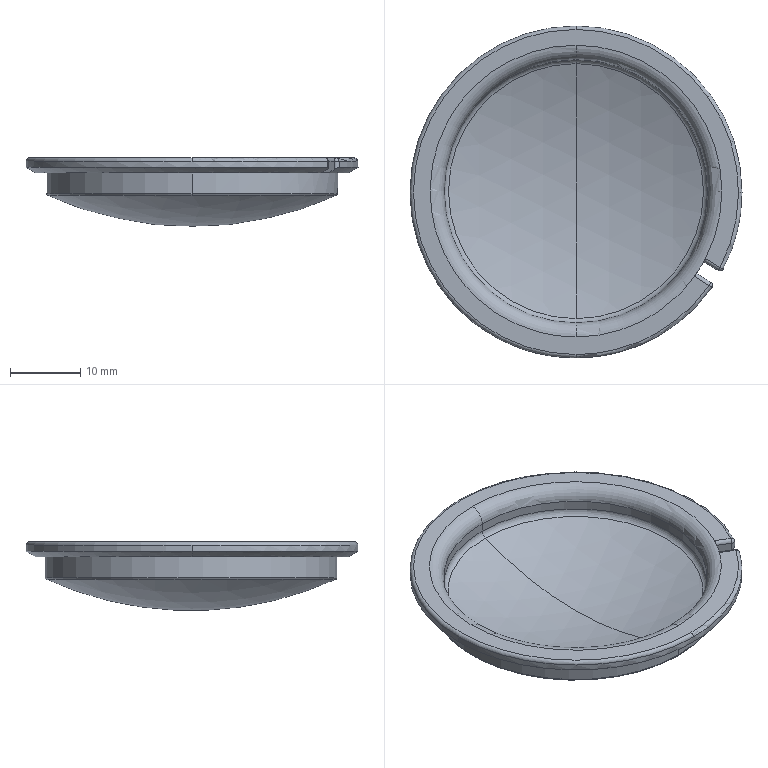Part | SolidWorks | features BaseBody 1 | 1 solid | 32 faces | box 47.34 x 47.34 x 9.8 mm | volume 4402 mm3 | torus 12 | cylinder 11 | sphere 5 | plane 4 | commonest cylinder face diameters 1 x4 47.34 x3 37.6 x2 41.6 x2
STEP:
#1=CARTESIAN_POINT('',(-125.381,28.46,-0.4856));
#2=VERTEX_POINT('',#1);
#3=CARTESIAN_POINT('',(-125.381,-12.906,-0.4856));
#4=VERTEX_POINT('',#3);
#5=CARTESIAN_POINT('',(-125.381,7.777,-0.4856));
#6=DIRECTION('',(0.,0.,-1.));
#7=DIRECTION('',(0.,-1.,0.));
#8=AXIS2_PLACEMENT_3D('',#5,#6,#7);
#9=CIRCLE('',#8,20.683);
#10=EDGE_CURVE('',#2,#4,#9,.T.);
#11=ORIENTED_EDGE('',*,*,#10,.F.);
#12=CARTESIAN_POINT('',(-125.381,28.577,-0.3035));
#13=VERTEX_POINT('',#12);
#14=CARTESIAN_POINT('',(-125.381,28.377,-0.3035));
#15=DIRECTION('',(1.,0.,0.));
#16=DIRECTION('',(0.,1.,0.));
#17=AXIS2_PLACEMENT_3D('',#14,#15,#16);
#18=CIRCLE('',#17,0.2);
#19=EDGE_CURVE('',#2,#13,#18,.T.);
#20=ORIENTED_EDGE('',*,*,#19,.T.);
#21=CARTESIAN_POINT('',(-125.381,-13.023,-0.3035));
#22=VERTEX_POINT('',#21);
#23=CARTESIAN_POINT('',(-125.381,7.777,-0.3035));
#24=DIRECTION('',(0.,0.,-1.));
#25=DIRECTION('',(0.,1.,0.));
#26=AXIS2_PLACEMENT_3D('',#23,#24,#25);
#27=CIRCLE('',#26,20.8);
#28=EDGE_CURVE('',#13,#22,#27,.T.);
#29=ORIENTED_EDGE('',*,*,#28,.T.);
#30=CARTESIAN_POINT('',(-125.381,-12.823,-0.3035));
#31=DIRECTION('',(-1.,0.,0.));
#32=DIRECTION('',(0.,0.,1.));
#33=AXIS2_PLACEMENT_3D('',#30,#31,#32);
#34=CIRCLE('',#33,0.2);
#35=EDGE_CURVE('',#4,#22,#34,.T.);
#36=ORIENTED_EDGE('',*,*,#35,.F.);
#37=EDGE_LOOP('',(#11,#20,#29,#36));
#38=FACE_OUTER_BOUND('',#37,.T.);
#39=CARTESIAN_POINT('',(-125.381,7.777,-0.3035));
#40=DIRECTION('',(0.,0.,1.));
#41=DIRECTION('',(0.,-1.,0.));
#42=AXIS2_PLACEMENT_3D('',#39,#40,#41);
#43=TOROIDAL_SURFACE('',#42,20.6,0.2);
#44=ADVANCED_FACE('',(#38),#43,.T.);
#45=ORIENTED_EDGE('',*,*,#28,.F.);
#46=CARTESIAN_POINT('',(-125.381,28.577,2.679));
#47=VERTEX_POINT('',#46);
#48=CARTESIAN_POINT('',(-125.381,28.577,-4.965));
#49=DIRECTION('',(0.,0.,1.));
#50=VECTOR('',#49,1000.);
#51=LINE('',#48,#50);
#52=EDGE_CURVE('',#13,#47,#51,.T.);
#53=ORIENTED_EDGE('',*,*,#52,.T.);
#54=CARTESIAN_POINT('',(-107.167,-2.268,2.679));
#55=VERTEX_POINT('',#54);
#56=CARTESIAN_POINT('',(-125.381,7.777,2.679));
#57=DIRECTION('',(0.,0.,-1.));
#58=DIRECTION('',(0.,-1.,0.));
#59=AXIS2_PLACEMENT_3D('',#56,#57,#58);
#60=CIRCLE('',#59,20.8);
#61=EDGE_CURVE('',#47,#55,#60,.T.);
#62=ORIENTED_EDGE('',*,*,#61,.T.);
#63=CARTESIAN_POINT('',(-107.167,-2.268,4.336));
#64=VERTEX_POINT('',#63);
#65=CARTESIAN_POINT('',(-107.167,-2.268,16.89));
#66=DIRECTION('',(0.,0.,1.));
#67=VECTOR('',#66,1000.);
#68=LINE('',#65,#67);
#69=EDGE_CURVE('',#55,#64,#68,.T.);
#70=ORIENTED_EDGE('',*,*,#69,.T.);
#71=CARTESIAN_POINT('',(-106.931,-1.826,4.836));
#72=VERTEX_POINT('',#71);
#73=CARTESIAN_POINT('',(-106.931,-1.826,4.836));
#74=CARTESIAN_POINT('',(-106.992,-1.944,4.836));
#75=CARTESIAN_POINT('',(-107.053,-2.058,4.782));
#76=CARTESIAN_POINT('',(-107.141,-2.22,4.598));
#77=CARTESIAN_POINT('',(-107.167,-2.268,4.468));
#78=CARTESIAN_POINT('',(-107.167,-2.268,4.336));
#79=B_SPLINE_CURVE_WITH_KNOTS('',3,(#73,#74,#75,#76,#77,#78),.UNSPECIFIED.,.F.,.F.,(4,2,4),(0.,0.0003909,0.0007818),.UNSPECIFIED.);
#80=EDGE_CURVE('',#72,#64,#79,.T.);
#81=ORIENTED_EDGE('',*,*,#80,.F.);
#82=CARTESIAN_POINT('',(-108.504,-4.381,4.836));
#83=VERTEX_POINT('',#82);
#84=CARTESIAN_POINT('',(-125.381,7.777,4.836));
#85=DIRECTION('',(0.,0.,-1.));
#86=DIRECTION('',(0.,-1.,0.));
#87=AXIS2_PLACEMENT_3D('',#84,#85,#86);
#88=CIRCLE('',#87,20.8);
#89=EDGE_CURVE('',#72,#83,#88,.T.);
#90=ORIENTED_EDGE('',*,*,#89,.T.);
#91=CARTESIAN_POINT('',(-108.216,-3.971,4.336));
#92=VERTEX_POINT('',#91);
#93=CARTESIAN_POINT('',(-108.216,-3.971,4.336));
#94=CARTESIAN_POINT('',(-108.216,-3.971,4.468));
#95=CARTESIAN_POINT('',(-108.247,-4.016,4.598));
#96=CARTESIAN_POINT('',(-108.352,-4.167,4.782));
#97=CARTESIAN_POINT('',(-108.427,-4.273,4.836));
#98=CARTESIAN_POINT('',(-108.504,-4.381,4.836));
#99=B_SPLINE_CURVE_WITH_KNOTS('',3,(#93,#94,#95,#96,#97,#98),.UNSPECIFIED.,.F.,.F.,(4,2,4),(0.,0.0003909,0.0007818),.UNSPECIFIED.);
#100=EDGE_CURVE('',#92,#83,#99,.T.);
#101=ORIENTED_EDGE('',*,*,#100,.F.);
#102=CARTESIAN_POINT('',(-108.216,-3.971,2.679));
#103=VERTEX_POINT('',#102);
#104=CARTESIAN_POINT('',(-108.216,-3.971,16.89));
#105=DIRECTION('',(0.,0.,-1.));
#106=VECTOR('',#105,1000.);
#107=LINE('',#104,#106);
#108=EDGE_CURVE('',#92,#103,#107,.T.);
#109=ORIENTED_EDGE('',*,*,#108,.T.);
#110=CARTESIAN_POINT('',(-125.381,-13.023,2.679));
#111=VERTEX_POINT('',#110);
#112=CARTESIAN_POINT('',(-125.381,7.777,2.679));
#113=DIRECTION('',(0.,0.,-1.));
#114=DIRECTION('',(0.,-1.,0.));
#115=AXIS2_PLACEMENT_3D('',#112,#113,#114);
#116=CIRCLE('',#115,20.8);
#117=EDGE_CURVE('',#103,#111,#116,.T.);
#118=ORIENTED_EDGE('',*,*,#117,.T.);
#119=CARTESIAN_POINT('',(-125.381,-13.023,-4.965));
#120=DIRECTION('',(0.,0.,1.));
#121=VECTOR('',#120,1000.);
#122=LINE('',#119,#121);
#123=EDGE_CURVE('',#22,#111,#122,.T.);
#124=ORIENTED_EDGE('',*,*,#123,.F.);
#125=EDGE_LOOP('',(#45,#53,#62,#70,#81,#90,#101,#109,#118,#124));
#126=FACE_OUTER_BOUND('',#125,.T.);
#127=CARTESIAN_POINT('',(-125.381,7.777,-4.965));
#128=DIRECTION('',(0.,0.,1.));
#129=DIRECTION('',(0.,-1.,0.));
#130=AXIS2_PLACEMENT_3D('',#127,#128,#129);
#131=CYLINDRICAL_SURFACE('',#130,20.8);
#132=ADVANCED_FACE('',(#126),#131,.T.);
#133=CARTESIAN_POINT('',(-149.051,7.647,3.467));
#134=VERTEX_POINT('',#133);
#135=CARTESIAN_POINT('',(-101.711,7.647,3.467));
#136=VERTEX_POINT('',#135);
#137=CARTESIAN_POINT('',(-125.381,7.647,3.467));
#138=DIRECTION('',(0.,0.,-1.));
#139=DIRECTION('',(-1.,0.,0.));
#140=AXIS2_PLACEMENT_3D('',#137,#138,#139);
#141=CIRCLE('',#140,23.67);
#142=EDGE_CURVE('',#134,#136,#141,.T.);
#143=ORIENTED_EDGE('',*,*,#142,.T.);
#144=CARTESIAN_POINT('',(-103.144,7.647,2.679));
#145=VERTEX_POINT('',#144);
#146=CARTESIAN_POINT('',(-125.511,7.647,45.036));
#147=DIRECTION('',(0.,1.,0.));
#148=DIRECTION('',(0.,0.,1.));
#149=AXIS2_PLACEMENT_3D('',#146,#147,#148);
#150=CIRCLE('',#149,47.9);
#151=EDGE_CURVE('',#136,#145,#150,.T.);
#152=ORIENTED_EDGE('',*,*,#151,.T.);
#153=CARTESIAN_POINT('',(-147.618,7.647,2.679));
#154=VERTEX_POINT('',#153);
#155=CARTESIAN_POINT('',(-125.381,7.647,2.679));
#156=DIRECTION('',(0.,0.,-1.));
#157=DIRECTION('',(-1.,0.,0.));
#158=AXIS2_PLACEMENT_3D('',#155,#156,#157);
#159=CIRCLE('',#158,22.237);
#160=EDGE_CURVE('',#154,#145,#159,.T.);
#161=ORIENTED_EDGE('',*,*,#160,.F.);
#162=CARTESIAN_POINT('',(-125.251,7.647,45.036));
#163=DIRECTION('',(0.,-1.,0.));
#164=DIRECTION('',(0.,0.,-1.));
#165=AXIS2_PLACEMENT_3D('',#162,#163,#164);
#166=CIRCLE('',#165,47.9);
#167=EDGE_CURVE('',#134,#154,#166,.T.);
#168=ORIENTED_EDGE('',*,*,#167,.F.);
#169=EDGE_LOOP('',(#143,#152,#161,#168));
#170=FACE_OUTER_BOUND('',#169,.T.);
#171=CARTESIAN_POINT('',(-125.381,7.647,45.036));
#172=DIRECTION('',(0.,0.,-1.));
#173=DIRECTION('',(-1.,0.,0.));
#174=AXIS2_PLACEMENT_3D('',#171,#172,#173);
#175=TOROIDAL_SURFACE('',#174,-0.1299,47.9);
#176=ADVANCED_FACE('',(#170),#175,.T.);
#177=CARTESIAN_POINT('',(-106.008,-5.953,3.467));
#178=VERTEX_POINT('',#177);
#179=CARTESIAN_POINT('',(-125.381,7.647,3.467));
#180=DIRECTION('',(0.,0.,-1.));
#181=DIRECTION('',(-1.,0.,0.));
#182=AXIS2_PLACEMENT_3D('',#179,#180,#181);
#183=CIRCLE('',#182,23.67);
#184=EDGE_CURVE('',#178,#134,#183,.T.);
#185=ORIENTED_EDGE('',*,*,#184,.T.);
#186=ORIENTED_EDGE('',*,*,#167,.T.);
#187=CARTESIAN_POINT('',(-106.929,-4.764,2.679));
#188=VERTEX_POINT('',#187);
#189=CARTESIAN_POINT('',(-125.381,7.647,2.679));
#190=DIRECTION('',(0.,0.,-1.));
#191=DIRECTION('',(-1.,0.,0.));
#192=AXIS2_PLACEMENT_3D('',#189,#190,#191);
#193=CIRCLE('',#192,22.237);
#194=EDGE_CURVE('',#188,#154,#193,.T.);
#195=ORIENTED_EDGE('',*,*,#194,.F.);
#196=CARTESIAN_POINT('',(-106.155,-5.24,3.171));
#197=VERTEX_POINT('',#196);
#198=CARTESIAN_POINT('',(-106.929,-4.764,2.679));
#199=CARTESIAN_POINT('',(-106.675,-4.92,2.836));
#200=CARTESIAN_POINT('',(-106.417,-5.079,3.));
#201=CARTESIAN_POINT('',(-106.155,-5.24,3.171));
#202=B_SPLINE_CURVE_WITH_KNOTS('',3,(#198,#199,#200,#201),.UNSPECIFIED.,.F.,.F.,(4,4),(0.,1.),.UNSPECIFIED.);
#203=EDGE_CURVE('',#188,#197,#202,.T.);
#204=ORIENTED_EDGE('',*,*,#203,.T.);
#205=CARTESIAN_POINT('',(-106.155,-5.24,3.171));
#206=CARTESIAN_POINT('',(-106.1,-5.274,3.207));
#207=CARTESIAN_POINT('',(-106.054,-5.317,3.242));
#208=CARTESIAN_POINT('',(-105.977,-5.421,3.311));
#209=CARTESIAN_POINT('',(-105.948,-5.481,3.343));
#210=CARTESIAN_POINT('',(-105.916,-5.612,3.4));
#211=CARTESIAN_POINT('',(-105.913,-5.682,3.424));
#212=CARTESIAN_POINT('',(-105.938,-5.824,3.458));
#213=CARTESIAN_POINT('',(-105.966,-5.892,3.467));
#214=CARTESIAN_POINT('',(-106.008,-5.953,3.467));
#215=B_SPLINE_CURVE_WITH_KNOTS('',3,(#205,#206,#207,#208,#209,#210,#211,#212,#213,#214),.UNSPECIFIED.,.F.,.F.,(4,2,2,2,4),(0.,0.0002173,0.0004346,0.000652,0.0008693),.UNSPECIFIED.);
#216=EDGE_CURVE('',#197,#178,#215,.T.);
#217=ORIENTED_EDGE('',*,*,#216,.T.);
#218=EDGE_LOOP('',(#185,#186,#195,#204,#217));
#219=FACE_OUTER_BOUND('',#218,.T.);
#220=CARTESIAN_POINT('',(-125.381,7.647,45.036));
#221=DIRECTION('',(0.,0.,-1.));
#222=DIRECTION('',(-1.,0.,0.));
#223=AXIS2_PLACEMENT_3D('',#220,#221,#222);
#224=TOROIDAL_SURFACE('',#223,-0.1299,47.9);
#225=ADVANCED_FACE('',(#219),#224,.T.);
#226=CARTESIAN_POINT('',(-125.381,26.577,2.836));
#227=VERTEX_POINT('',#226);
#228=CARTESIAN_POINT('',(-125.381,-11.023,2.836));
#229=VERTEX_POINT('',#228);
#230=CARTESIAN_POINT('',(-125.381,7.777,2.836));
#231=DIRECTION('',(0.,0.,-1.));
#232=DIRECTION('',(0.,1.,0.));
#233=AXIS2_PLACEMENT_3D('',#230,#231,#232);
#234=CIRCLE('',#233,18.8);
#235=EDGE_CURVE('',#227,#229,#234,.T.);
#236=ORIENTED_EDGE('',*,*,#235,.T.);
#237=CARTESIAN_POINT('',(-125.381,-13.023,4.836));
#238=VERTEX_POINT('',#237);
#239=CARTESIAN_POINT('',(-125.381,-13.023,2.836));
#240=DIRECTION('',(1.,0.,0.));
#241=DIRECTION('',(0.,1.,0.));
#242=AXIS2_PLACEMENT_3D('',#239,#240,#241);
#243=CIRCLE('',#242,2.);
#244=EDGE_CURVE('',#229,#238,#243,.T.);
#245=ORIENTED_EDGE('',*,*,#244,.T.);
#246=CARTESIAN_POINT('',(-125.381,-13.023,4.836));
#247=CARTESIAN_POINT('',(-124.572,-13.023,4.836));
#248=CARTESIAN_POINT('',(-123.763,-12.976,4.836));
#249=CARTESIAN_POINT('',(-122.559,-12.835,4.836));
#250=CARTESIAN_POINT('',(-122.159,-12.777,4.836));
#251=CARTESIAN_POINT('',(-121.562,-12.671,4.836));
#252=CARTESIAN_POINT('',(-121.314,-12.623,4.836));
#253=CARTESIAN_POINT('',(-121.055,-12.568,4.836));
#254=CARTESIAN_POINT('',(-120.993,-12.555,4.836));
#255=CARTESIAN_POINT('',(-120.978,-12.552,4.836));
#256=CARTESIAN_POINT('',(-120.978,-12.552,4.836));
#257=CARTESIAN_POINT('',(-120.977,-12.551,4.836));
#258=CARTESIAN_POINT('',(-120.974,-12.551,4.836));
#259=CARTESIAN_POINT('',(-120.964,-12.549,4.836));
#260=CARTESIAN_POINT('',(-120.92,-12.539,4.836));
#261=CARTESIAN_POINT('',(-120.857,-12.525,4.836));
#262=CARTESIAN_POINT('',(-120.537,-12.453,4.836));
#263=CARTESIAN_POINT('',(-120.066,-12.345,4.836));
#264=CARTESIAN_POINT('',(-119.38,-12.139,4.836));
#265=CARTESIAN_POINT('',(-119.369,-12.136,4.836));
#266=CARTESIAN_POINT('',(-119.348,-12.129,4.836));
#267=CARTESIAN_POINT('',(-119.335,-12.125,4.836));
#268=CARTESIAN_POINT('',(-119.315,-12.119,4.836));
#269=CARTESIAN_POINT('',(-119.274,-12.107,4.836));
#270=CARTESIAN_POINT('',(-119.178,-12.077,4.836));
#271=CARTESIAN_POINT('',(-118.991,-12.018,4.836));
#272=CARTESIAN_POINT('',(-118.835,-11.967,4.836));
#273=CARTESIAN_POINT('',(-118.531,-11.864,4.836));
#274=CARTESIAN_POINT('',(-118.336,-11.795,4.836));
#275=CARTESIAN_POINT('',(-118.057,-11.692,4.836));
#276=CARTESIAN_POINT('',(-117.921,-11.64,4.836));
#277=CARTESIAN_POINT('',(-117.789,-11.589,4.836));
#278=CARTESIAN_POINT('',(-117.735,-11.567,4.836));
#279=CARTESIAN_POINT('',(-117.727,-11.564,4.836));
#280=CARTESIAN_POINT('',(-117.693,-11.55,4.836));
#281=CARTESIAN_POINT('',(-117.642,-11.53,4.836));
#282=CARTESIAN_POINT('',(-117.326,-11.403,4.836));
#283=CARTESIAN_POINT('',(-117.047,-11.283,4.836));
#284=CARTESIAN_POINT('',(-116.35,-10.967,4.836));
#285=CARTESIAN_POINT('',(-115.949,-10.766,4.836));
#286=CARTESIAN_POINT('',(-115.262,-10.4,4.836));
#287=CARTESIAN_POINT('',(-114.978,-10.237,4.836));
#288=CARTESIAN_POINT('',(-114.719,-10.083,4.836));
#289=CARTESIAN_POINT('',(-114.688,-10.064,4.836));
#290=CARTESIAN_POINT('',(-114.657,-10.046,4.836));
#291=CARTESIAN_POINT('',(-114.651,-10.042,4.836));
#292=CARTESIAN_POINT('',(-114.644,-10.038,4.836));
#293=CARTESIAN_POINT('',(-114.628,-10.028,4.836));
#294=CARTESIAN_POINT('',(-114.595,-10.008,4.836));
#295=CARTESIAN_POINT('',(-114.474,-9.935,4.836));
#296=CARTESIAN_POINT('',(-114.191,-9.759,4.836));
#297=CARTESIAN_POINT('',(-113.758,-9.477,4.836));
#298=CARTESIAN_POINT('',(-113.33,-9.179,4.836));
#299=CARTESIAN_POINT('',(-113.055,-8.978,4.836));
#300=CARTESIAN_POINT('',(-112.939,-8.892,4.836));
#301=CARTESIAN_POINT('',(-112.907,-8.868,4.836));
#302=CARTESIAN_POINT('',(-112.891,-8.856,4.836));
#303=CARTESIAN_POINT('',(-112.887,-8.853,4.836));
#304=CARTESIAN_POINT('',(-112.873,-8.843,4.836));
#305=CARTESIAN_POINT('',(-112.812,-8.797,4.836));
#306=CARTESIAN_POINT('',(-112.753,-8.752,4.836));
#307=CARTESIAN_POINT('',(-112.288,-8.394,4.836));
#308=CARTESIAN_POINT('',(-111.947,-8.107,4.836));
#309=CARTESIAN_POINT('',(-111.53,-7.742,4.836));
#310=CARTESIAN_POINT('',(-111.407,-7.631,4.836));
#311=CARTESIAN_POINT('',(-111.286,-7.519,4.836));
#312=CARTESIAN_POINT('',(-111.272,-7.507,4.836));
#313=CARTESIAN_POINT('',(-111.253,-7.488,4.836));
#314=CARTESIAN_POINT('',(-111.243,-7.48,4.836));
#315=CARTESIAN_POINT('',(-111.224,-7.462,4.836));
#316=CARTESIAN_POINT('',(-111.178,-7.419,4.836));
#317=CARTESIAN_POINT('',(-111.058,-7.307,4.836));
#318=CARTESIAN_POINT('',(-110.657,-6.923,4.836));
#319=CARTESIAN_POINT('',(-110.305,-6.56,4.836));
#320=CARTESIAN_POINT('',(-109.487,-5.665,4.836));
#321=CARTESIAN_POINT('',(-108.976,-5.037,4.836));
#322=CARTESIAN_POINT('',(-108.504,-4.381,4.836));
#323=B_SPLINE_CURVE_WITH_KNOTS('',3,(#246,#247,#248,#249,#250,#251,#252,#253,#254,#255,#256,#257,#258,#259,#260,#261,#262,#263,#264,#265,#266,#267,#268,#269,#270,#271,#272,#273,#274,#275,#276,#277,#278,#279,#280,#281,#282,#283,#284,#285,#286,#287,#288,#289,#290,#291,#292,#293,#294,#295,#296,#297,#298,#299,#300,#301,#302,#303,#304,#305,#306,#307,#308,#309,#310,#311,#312,#313,#314,#315,#316,#317,#318,#319,#320,#321,#322),.UNSPECIFIED.,.F.,.F.,(4,2,2,1,1,2,2,1,1,1,2,2,2,2,1,1,1,2,2,1,2,2,1,1,2,2,2,1,2,2,1,1,1,1,1,1,1,2,2,1,2,2,2,2,2,1,1,1,2,4),(0.,0.125,0.1875,0.2188,0.2266,0.2285,0.229,0.2295,0.2305,0.2344,0.25,0.3125,0.3135,0.3145,0.3164,0.3203,0.3281,0.3438,0.375,0.3906,0.3984,0.4004,0.4023,0.4063,0.4375,0.5,0.5625,0.5703,0.5713,0.5723,0.5742,0.5781,0.5938,0.625,0.6563,0.6719,0.6758,0.6777,0.6787,0.6797,0.6875,0.75,0.7813,0.7852,0.7871,0.7891,0.7969,0.8125,0.875,1.),.UNSPECIFIED.);
#324=EDGE_CURVE('',#238,#83,#323,.T.);
#325=ORIENTED_EDGE('',*,*,#324,.T.);
#326=ORIENTED_EDGE('',*,*,#89,.F.);
#327=CARTESIAN_POINT('',(-125.381,28.577,4.836));
#328=VERTEX_POINT('',#327);
#329=CARTESIAN_POINT('',(-125.381,7.777,4.836));
#330=DIRECTION('',(0.,0.,1.));
#331=DIRECTION('',(0.,1.,0.));
#332=AXIS2_PLACEMENT_3D('',#329,#330,#331);
#333=CIRCLE('',#332,20.8);
#334=EDGE_CURVE('',#72,#328,#333,.T.);
#335=ORIENTED_EDGE('',*,*,#334,.T.);
#336=CARTESIAN_POINT('',(-125.381,28.577,2.836));
#337=DIRECTION('',(-1.,0.,0.));
#338=DIRECTION('',(0.,0.,1.));
#339=AXIS2_PLACEMENT_3D('',#336,#337,#338);
#340=CIRCLE('',#339,2.);
#341=EDGE_CURVE('',#227,#328,#340,.T.);
#342=ORIENTED_EDGE('',*,*,#341,.F.);
#343=EDGE_LOOP('',(#236,#245,#325,#326,#335,#342));
#344=FACE_OUTER_BOUND('',#343,.T.);
#345=CARTESIAN_POINT('',(-125.381,7.777,2.836));
#346=DIRECTION('',(0.,0.,-1.));
#347=DIRECTION('',(0.,1.,0.));
#348=AXIS2_PLACEMENT_3D('',#345,#346,#347);
#349=TOROIDAL_SURFACE('',#348,20.8,2.);
#350=ADVANCED_FACE('',(#344),#349,.T.);
#351=CARTESIAN_POINT('',(-125.381,31.317,4.336));
#352=VERTEX_POINT('',#351);
#353=CARTESIAN_POINT('',(-101.711,7.647,4.336));
#354=VERTEX_POINT('',#353);
#355=CARTESIAN_POINT('',(-125.381,7.647,4.336));
#356=DIRECTION('',(0.,0.,-1.));
#357=DIRECTION('',(-1.,0.,0.));
#358=AXIS2_PLACEMENT_3D('',#355,#356,#357);
#359=CIRCLE('',#358,23.67);
#360=EDGE_CURVE('',#352,#354,#359,.T.);
#361=ORIENTED_EDGE('',*,*,#360,.T.);
#362=CARTESIAN_POINT('',(-101.711,7.647,-4.5));
#363=DIRECTION('',(0.,0.,-1.));
#364=VECTOR('',#363,1000.);
#365=LINE('',#362,#364);
#366=EDGE_CURVE('',#354,#136,#365,.T.);
#367=ORIENTED_EDGE('',*,*,#366,.T.);
#368=ORIENTED_EDGE('',*,*,#142,.F.);
#369=CARTESIAN_POINT('',(-149.051,7.647,4.336));
#370=VERTEX_POINT('',#369);
#371=CARTESIAN_POINT('',(-149.051,7.647,-4.5));
#372=DIRECTION('',(0.,0.,-1.));
#373=VECTOR('',#372,1000.);
#374=LINE('',#371,#373);
#375=EDGE_CURVE('',#370,#134,#374,.T.);
#376=ORIENTED_EDGE('',*,*,#375,.F.);
#377=CARTESIAN_POINT('',(-125.381,7.647,4.336));
#378=DIRECTION('',(0.,0.,-1.));
#379=DIRECTION('',(-1.,0.,0.));
#380=AXIS2_PLACEMENT_3D('',#377,#378,#379);
#381=CIRCLE('',#380,23.67);
#382=EDGE_CURVE('',#370,#352,#381,.T.);
#383=ORIENTED_EDGE('',*,*,#382,.T.);
#384=EDGE_LOOP('',(#361,#367,#368,#376,#383));
#385=FACE_OUTER_BOUND('',#384,.T.);
#386=CARTESIAN_POINT('',(-125.381,7.647,-4.5));
#387=DIRECTION('',(0.,0.,-1.));
#388=DIRECTION('',(-1.,0.,0.));
#389=AXIS2_PLACEMENT_3D('',#386,#387,#388);
#390=CYLINDRICAL_SURFACE('',#389,23.67);
#391=ADVANCED_FACE('',(#385),#390,.T.);
#392=CARTESIAN_POINT('',(-125.381,-16.023,4.336));
#393=VERTEX_POINT('',#392);
#394=CARTESIAN_POINT('',(-125.381,7.647,4.336));
#395=DIRECTION('',(0.,0.,-1.));
#396=DIRECTION('',(-1.,0.,0.));
#397=AXIS2_PLACEMENT_3D('',#394,#395,#396);
#398=CIRCLE('',#397,23.67);
#399=EDGE_CURVE('',#393,#370,#398,.T.);
#400=ORIENTED_EDGE('',*,*,#399,.T.);
#401=ORIENTED_EDGE('',*,*,#375,.T.);
#402=ORIENTED_EDGE('',*,*,#184,.F.);
#403=CARTESIAN_POINT('',(-106.008,-5.953,4.336));
#404=VERTEX_POINT('',#403);
#405=CARTESIAN_POINT('',(-106.008,-5.953,-4.5));
#406=DIRECTION('',(0.,0.,1.));
#407=VECTOR('',#406,1000.);
#408=LINE('',#405,#407);
#409=EDGE_CURVE('',#178,#404,#408,.T.);
#410=ORIENTED_EDGE('',*,*,#409,.T.);
#411=CARTESIAN_POINT('',(-125.381,7.647,4.336));
#412=DIRECTION('',(0.,0.,-1.));
#413=DIRECTION('',(-1.,0.,0.));
#414=AXIS2_PLACEMENT_3D('',#411,#412,#413);
#415=CIRCLE('',#414,23.67);
#416=EDGE_CURVE('',#404,#393,#415,.T.);
#417=ORIENTED_EDGE('',*,*,#416,.T.);
#418=EDGE_LOOP('',(#400,#401,#402,#410,#417));
#419=FACE_OUTER_BOUND('',#418,.T.);
#420=CARTESIAN_POINT('',(-125.381,7.647,-4.5));
#421=DIRECTION('',(0.,0.,-1.));
#422=DIRECTION('',(-1.,0.,0.));
#423=AXIS2_PLACEMENT_3D('',#420,#421,#422);
#424=CYLINDRICAL_SURFACE('',#423,23.67);
#425=ADVANCED_FACE('',(#419),#424,.T.);
#426=CARTESIAN_POINT('',(-125.381,26.577,1.537));
#427=VERTEX_POINT('',#426);
#428=CARTESIAN_POINT('',(-125.381,-11.023,1.537));
#429=VERTEX_POINT('',#428);
#430=CARTESIAN_POINT('',(-125.381,7.777,1.537));
#431=DIRECTION('',(0.,0.,1.));
#432=DIRECTION('',(0.,-1.,0.));
#433=AXIS2_PLACEMENT_3D('',#430,#431,#432);
#434=CIRCLE('',#433,18.8);
#435=EDGE_CURVE('',#427,#429,#434,.T.);
#436=ORIENTED_EDGE('',*,*,#435,.F.);
#437=CARTESIAN_POINT('',(-125.381,26.577,-4.965));
#438=DIRECTION('',(0.,0.,1.));
#439=VECTOR('',#438,1000.);
#440=LINE('',#437,#439);
#441=EDGE_CURVE('',#427,#227,#440,.T.);
#442=ORIENTED_EDGE('',*,*,#441,.T.);
#443=CARTESIAN_POINT('',(-125.381,7.777,2.836));
#444=DIRECTION('',(0.,0.,-1.));
#445=DIRECTION('',(0.,1.,0.));
#446=AXIS2_PLACEMENT_3D('',#443,#444,#445);
#447=CIRCLE('',#446,18.8);
#448=EDGE_CURVE('',#229,#227,#447,.T.);
#449=ORIENTED_EDGE('',*,*,#448,.F.);
#450=CARTESIAN_POINT('',(-125.381,-11.023,-4.965));
#451=DIRECTION('',(0.,0.,1.));
#452=VECTOR('',#451,1000.);
#453=LINE('',#450,#452);
#454=EDGE_CURVE('',#429,#229,#453,.T.);
#455=ORIENTED_EDGE('',*,*,#454,.F.);
#456=EDGE_LOOP('',(#436,#442,#449,#455));
#457=FACE_OUTER_BOUND('',#456,.T.);
#458=CARTESIAN_POINT('',(-125.381,7.777,-4.965));
#459=DIRECTION('',(0.,0.,1.));
#460=DIRECTION('',(0.,-1.,0.));
#461=AXIS2_PLACEMENT_3D('',#458,#459,#460);
#462=CYLINDRICAL_SURFACE('',#461,18.8);
#463=ADVANCED_FACE('',(#457),#462,.F.);
#464=CARTESIAN_POINT('',(-106.418,-5.666,4.836));
#465=VERTEX_POINT('',#464);
#466=CARTESIAN_POINT('',(-125.381,-15.523,4.836));
#467=VERTEX_POINT('',#466);
#468=CARTESIAN_POINT('',(-106.418,-5.666,4.836));
#469=CARTESIAN_POINT('',(-106.942,-6.412,4.836));
#470=CARTESIAN_POINT('',(-107.509,-7.128,4.836));
#471=CARTESIAN_POINT('',(-108.422,-8.148,4.836));
#472=CARTESIAN_POINT('',(-108.736,-8.479,4.836));
#473=CARTESIAN_POINT('',(-109.222,-8.96,4.836));
#474=CARTESIAN_POINT('',(-109.468,-9.198,4.836));
#475=CARTESIAN_POINT('',(-109.762,-9.468,4.836));
#476=CARTESIAN_POINT('',(-109.91,-9.601,4.836));
#477=CARTESIAN_POINT('',(-109.984,-9.668,4.836));
#478=CARTESIAN_POINT('',(-110.022,-9.701,4.836));
#479=CARTESIAN_POINT('',(-110.04,-9.717,4.836));
#480=CARTESIAN_POINT('',(-110.05,-9.725,4.836));
#481=CARTESIAN_POINT('',(-110.054,-9.729,4.836));
#482=CARTESIAN_POINT('',(-110.056,-9.731,4.836));
#483=CARTESIAN_POINT('',(-110.059,-9.734,4.836));
#484=CARTESIAN_POINT('',(-110.082,-9.754,4.836));
#485=CARTESIAN_POINT('',(-110.181,-9.842,4.836));
#486=CARTESIAN_POINT('',(-110.45,-10.071,4.836));
#487=CARTESIAN_POINT('',(-110.559,-10.163,4.836));
#488=CARTESIAN_POINT('',(-110.755,-10.324,4.836));
#489=CARTESIAN_POINT('',(-110.825,-10.381,4.836));
#490=CARTESIAN_POINT('',(-110.939,-10.472,4.836));
#491=CARTESIAN_POINT('',(-110.998,-10.519,4.836));
#492=CARTESIAN_POINT('',(-111.07,-10.576,4.836));
#493=CARTESIAN_POINT('',(-111.107,-10.605,4.836));
#494=CARTESIAN_POINT('',(-111.126,-10.62,4.836));
#495=CARTESIAN_POINT('',(-111.134,-10.626,4.836));
#496=CARTESIAN_POINT('',(-111.14,-10.63,4.836));
#497=CARTESIAN_POINT('',(-111.143,-10.633,4.836));
#498=CARTESIAN_POINT('',(-111.359,-10.801,4.836));
#499=CARTESIAN_POINT('',(-111.561,-10.952,4.836));
#500=CARTESIAN_POINT('',(-111.845,-11.159,4.836));
#501=CARTESIAN_POINT('',(-111.937,-11.225,4.836));
#502=CARTESIAN_POINT('',(-112.069,-11.318,4.836));
#503=CARTESIAN_POINT('',(-112.134,-11.363,4.836));
#504=CARTESIAN_POINT('',(-112.208,-11.414,4.836));
#505=CARTESIAN_POINT('',(-112.244,-11.439,4.836));
#506=CARTESIAN_POINT('',(-112.259,-11.45,4.836));
#507=CARTESIAN_POINT('',(-112.27,-11.457,4.836));
#508=CARTESIAN_POINT('',(-112.274,-11.46,4.836));
#509=CARTESIAN_POINT('',(-112.667,-11.73,4.836));
#510=CARTESIAN_POINT('',(-113.063,-11.983,4.836));
#511=CARTESIAN_POINT('',(-113.667,-12.345,4.836));
#512=CARTESIAN_POINT('',(-113.972,-12.522,4.836));
#513=CARTESIAN_POINT('',(-114.332,-12.719,4.836));
#514=CARTESIAN_POINT('',(-114.513,-12.816,4.836));
#515=CARTESIAN_POINT('',(-114.604,-12.864,4.836));
#516=CARTESIAN_POINT('',(-114.649,-12.888,4.836));
#517=CARTESIAN_POINT('',(-114.672,-12.9,4.836));
#518=CARTESIAN_POINT('',(-114.683,-12.906,4.836));
#519=CARTESIAN_POINT('',(-114.688,-12.908,4.836));
#520=CARTESIAN_POINT('',(-114.692,-12.91,4.836));
#521=CARTESIAN_POINT('',(-114.695,-12.911,4.836));
#522=CARTESIAN_POINT('',(-114.735,-12.932,4.836));
#523=CARTESIAN_POINT('',(-114.858,-12.997,4.836));
#524=CARTESIAN_POINT('',(-115.174,-13.154,4.836));
#525=CARTESIAN_POINT('',(-115.301,-13.216,4.836));
#526=CARTESIAN_POINT('',(-115.525,-13.323,4.836));
#527=CARTESIAN_POINT('',(-115.605,-13.36,4.836));
#528=CARTESIAN_POINT('',(-115.734,-13.42,4.836));
#529=CARTESIAN_POINT('',(-115.801,-13.45,4.836));
#530=CARTESIAN_POINT('',(-115.882,-13.487,4.836));
#531=CARTESIAN_POINT('',(-115.924,-13.505,4.836));
#532=CARTESIAN_POINT('',(-115.945,-13.515,4.836));
#533=CARTESIAN_POINT('',(-115.954,-13.519,4.836));
#534=CARTESIAN_POINT('',(-115.96,-13.521,4.836));
#535=CARTESIAN_POINT('',(-115.964,-13.523,4.836));
#536=CARTESIAN_POINT('',(-116.213,-13.634,4.836));
#537=CARTESIAN_POINT('',(-116.446,-13.733,4.836));
#538=CARTESIAN_POINT('',(-116.771,-13.865,4.836));
#539=CARTESIAN_POINT('',(-116.928,-13.927,4.836));
#540=CARTESIAN_POINT('',(-117.101,-13.994,4.836));
#541=CARTESIAN_POINT('',(-117.185,-14.026,4.836));
#542=CARTESIAN_POINT('',(-117.226,-14.041,4.836));
#543=CARTESIAN_POINT('',(-117.244,-14.048,4.836));
#544=CARTESIAN_POINT('',(-117.255,-14.052,4.836));
#545=CARTESIAN_POINT('',(-117.26,-14.054,4.836));
#546=CARTESIAN_POINT('',(-117.707,-14.221,4.836));
#547=CARTESIAN_POINT('',(-118.152,-14.372,4.836));
#548=CARTESIAN_POINT('',(-118.825,-14.578,4.836));
#549=CARTESIAN_POINT('',(-119.163,-14.676,4.836));
#550=CARTESIAN_POINT('',(-119.561,-14.781,4.836));
#551=CARTESIAN_POINT('',(-119.76,-14.831,4.836));
#552=CARTESIAN_POINT('',(-119.86,-14.856,4.836));
#553=CARTESIAN_POINT('',(-119.909,-14.868,4.836));
#554=CARTESIAN_POINT('',(-119.934,-14.874,4.836));
#555=CARTESIAN_POINT('',(-119.947,-14.877,4.836));
#556=CARTESIAN_POINT('',(-119.952,-14.878,4.836));
#557=CARTESIAN_POINT('',(-119.956,-14.879,4.836));
#558=CARTESIAN_POINT('',(-119.959,-14.88,4.836));
#559=CARTESIAN_POINT('',(-120.,-14.89,4.836));
#560=CARTESIAN_POINT('',(-120.132,-14.922,4.836));
#561=CARTESIAN_POINT('',(-120.466,-14.996,4.836));
#562=CARTESIAN_POINT('',(-120.601,-15.025,4.836));
#563=CARTESIAN_POINT('',(-120.837,-15.073,4.836));
#564=CARTESIAN_POINT('',(-120.921,-15.09,4.836));
#565=CARTESIAN_POINT('',(-121.057,-15.116,4.836));
#566=CARTESIAN_POINT('',(-121.127,-15.129,4.836));
#567=CARTESIAN_POINT('',(-121.212,-15.145,4.836));
#568=CARTESIAN_POINT('',(-121.256,-15.153,4.836));
#569=CARTESIAN_POINT('',(-121.278,-15.157,4.836));
#570=CARTESIAN_POINT('',(-121.288,-15.159,4.836));
#571=CARTESIAN_POINT('',(-121.294,-15.16,4.836));
#572=CARTESIAN_POINT('',(-121.298,-15.161,4.836));
#573=CARTESIAN_POINT('',(-121.56,-15.208,4.836));
#574=CARTESIAN_POINT('',(-121.802,-15.247,4.836));
#575=CARTESIAN_POINT('',(-122.14,-15.296,4.836));
#576=CARTESIAN_POINT('',(-122.249,-15.311,4.836));
#577=CARTESIAN_POINT('',(-122.404,-15.332,4.836));
#578=CARTESIAN_POINT('',(-122.481,-15.341,4.836));
#579=CARTESIAN_POINT('',(-122.567,-15.352,4.836));
#580=CARTESIAN_POINT('',(-122.609,-15.357,4.836));
#581=CARTESIAN_POINT('',(-122.627,-15.359,4.836));
#582=CARTESIAN_POINT('',(-122.639,-15.361,4.836));
#583=CARTESIAN_POINT('',(-122.644,-15.361,4.836));
#584=CARTESIAN_POINT('',(-123.557,-15.47,4.836));
#585=CARTESIAN_POINT('',(-124.469,-15.523,4.836));
#586=CARTESIAN_POINT('',(-125.381,-15.523,4.836));
#587=B_SPLINE_CURVE_WITH_KNOTS('',3,(#468,#469,#470,#471,#472,#473,#474,#475,#476,#477,#478,#479,#480,#481,#482,#483,#484,#485,#486,#487,#488,#489,#490,#491,#492,#493,#494,#495,#496,#497,#498,#499,#500,#501,#502,#503,#504,#505,#506,#507,#508,#509,#510,#511,#512,#513,#514,#515,#516,#517,#518,#519,#520,#521,#522,#523,#524,#525,#526,#527,#528,#529,#530,#531,#532,#533,#534,#535,#536,#537,#538,#539,#540,#541,#542,#543,#544,#545,#546,#547,#548,#549,#550,#551,#552,#553,#554,#555,#556,#557,#558,#559,#560,#561,#562,#563,#564,#565,#566,#567,#568,#569,#570,#571,#572,#573,#574,#575,#576,#577,#578,#579,#580,#581,#582,#583,#584,#585,#586),.UNSPECIFIED.,.F.,.F.,(4,2,2,1,1,1,1,1,1,1,2,2,2,2,2,1,1,1,1,2,2,2,2,1,1,1,2,2,2,1,1,1,1,1,1,1,2,2,2,2,2,1,1,1,1,2,2,2,1,1,1,1,2,2,2,1,1,1,1,1,1,1,2,2,2,2,2,1,1,1,1,2,2,2,2,1,1,1,2,2,4),(0.,0.125,0.1875,0.2187,0.2344,0.2422,0.2461,0.248,0.249,0.2495,0.2498,0.25,0.2812,0.2969,0.3047,0.3086,0.3105,0.3115,0.312,0.3123,0.3125,0.3437,0.3594,0.3672,0.3711,0.373,0.374,0.375,0.4375,0.4687,0.4844,0.4922,0.4961,0.498,0.499,0.4995,0.4998,0.5,0.5312,0.5469,0.5547,0.5586,0.5605,0.5615,0.562,0.5623,0.5625,0.5937,0.6094,0.6172,0.6211,0.623,0.624,0.625,0.6875,0.7187,0.7344,0.7422,0.7461,0.748,0.749,0.7495,0.7498,0.75,0.7812,0.7969,0.8047,0.8086,0.8105,0.8115,0.812,0.8123,0.8125,0.8437,0.8594,0.8672,0.8711,0.873,0.874,0.875,1.),.UNSPECIFIED.);
#588=EDGE_CURVE('',#465,#467,#587,.T.);
#589=ORIENTED_EDGE('',*,*,#588,.T.);
#590=CARTESIAN_POINT('',(-125.381,-15.523,4.336));
#591=DIRECTION('',(1.,0.,0.));
#592=DIRECTION('',(0.,1.,0.));
#593=AXIS2_PLACEMENT_3D('',#590,#591,#592);
#594=CIRCLE('',#593,0.5);
#595=EDGE_CURVE('',#467,#393,#594,.T.);
#596=ORIENTED_EDGE('',*,*,#595,.T.);
#597=ORIENTED_EDGE('',*,*,#416,.F.);
#598=CARTESIAN_POINT('',(-106.418,-5.666,4.336));
#599=DIRECTION('',(-0.5746,-0.8185,0.));
#600=DIRECTION('',(0.8185,-0.5746,0.));
#601=AXIS2_PLACEMENT_3D('',#598,#599,#600);
#602=CIRCLE('',#601,0.5);
#603=EDGE_CURVE('',#404,#465,#602,.T.);
#604=ORIENTED_EDGE('',*,*,#603,.T.);
#605=EDGE_LOOP('',(#589,#596,#597,#604));
#606=FACE_OUTER_BOUND('',#605,.T.);
#607=CARTESIAN_POINT('',(-125.381,7.647,4.336));
#608=DIRECTION('',(0.,0.,-1.));
#609=DIRECTION('',(0.,1.,0.));
#610=AXIS2_PLACEMENT_3D('',#607,#608,#609);
#611=TOROIDAL_SURFACE('',#610,23.17,0.5);
#612=ADVANCED_FACE('',(#606),#611,.T.);
#613=ORIENTED_EDGE('',*,*,#595,.F.);
#614=CARTESIAN_POINT('',(-125.381,30.817,4.836));
#615=VERTEX_POINT('',#614);
#616=CARTESIAN_POINT('',(-125.381,7.647,4.836));
#617=DIRECTION('',(0.,0.,-1.));
#618=DIRECTION('',(0.,1.,0.));
#619=AXIS2_PLACEMENT_3D('',#616,#617,#618);
#620=CIRCLE('',#619,23.17);
#621=EDGE_CURVE('',#467,#615,#620,.T.);
#622=ORIENTED_EDGE('',*,*,#621,.T.);
#623=CARTESIAN_POINT('',(-125.381,30.817,4.336));
#624=DIRECTION('',(-1.,0.,0.));
#625=DIRECTION('',(0.,0.,1.));
#626=AXIS2_PLACEMENT_3D('',#623,#624,#625);
#627=CIRCLE('',#626,0.5);
#628=EDGE_CURVE('',#615,#352,#627,.T.);
#629=ORIENTED_EDGE('',*,*,#628,.T.);
#630=ORIENTED_EDGE('',*,*,#382,.F.);
#631=ORIENTED_EDGE('',*,*,#399,.F.);
#632=EDGE_LOOP('',(#613,#622,#629,#630,#631));
#633=FACE_OUTER_BOUND('',#632,.T.);
#634=CARTESIAN_POINT('',(-125.381,7.647,4.336));
#635=DIRECTION('',(0.,0.,-1.));
#636=DIRECTION('',(0.,1.,0.));
#637=AXIS2_PLACEMENT_3D('',#634,#635,#636);
#638=TOROIDAL_SURFACE('',#637,23.17,0.5);
#639=ADVANCED_FACE('',(#633),#638,.T.);
#640=CARTESIAN_POINT('',(-125.381,25.956,0.6116));
#641=VERTEX_POINT('',#640);
#642=CARTESIAN_POINT('',(-125.381,-10.402,0.6116));
#643=VERTEX_POINT('',#642);
#644=CARTESIAN_POINT('',(-125.381,7.777,0.6116));
#645=DIRECTION('',(0.,0.,1.));
#646=DIRECTION('',(0.,-1.,0.));
#647=AXIS2_PLACEMENT_3D('',#644,#645,#646);
#648=CIRCLE('',#647,18.179);
#649=EDGE_CURVE('',#641,#643,#648,.T.);
#650=ORIENTED_EDGE('',*,*,#649,.F.);
#651=CARTESIAN_POINT('',(-125.381,25.577,1.537));
#652=DIRECTION('',(1.,0.,0.));
#653=DIRECTION('',(0.,1.,0.));
#654=AXIS2_PLACEMENT_3D('',#651,#652,#653);
#655=CIRCLE('',#654,1.);
#656=EDGE_CURVE('',#641,#427,#655,.T.);
#657=ORIENTED_EDGE('',*,*,#656,.T.);
#658=ORIENTED_EDGE('',*,*,#435,.T.);
#659=CARTESIAN_POINT('',(-125.381,-10.023,1.537));
#660=DIRECTION('',(-1.,0.,0.));
#661=DIRECTION('',(0.,0.,1.));
#662=AXIS2_PLACEMENT_3D('',#659,#660,#661);
#663=CIRCLE('',#662,1.);
#664=EDGE_CURVE('',#643,#429,#663,.T.);
#665=ORIENTED_EDGE('',*,*,#664,.F.);
#666=EDGE_LOOP('',(#650,#657,#658,#665));
#667=FACE_OUTER_BOUND('',#666,.T.);
#668=CARTESIAN_POINT('',(-125.381,7.777,1.537));
#669=DIRECTION('',(0.,0.,1.));
#670=DIRECTION('',(0.,-1.,0.));
#671=AXIS2_PLACEMENT_3D('',#668,#669,#670);
#672=TOROIDAL_SURFACE('',#671,17.8,1.);
#673=ADVANCED_FACE('',(#667),#672,.F.);
#674=CARTESIAN_POINT('',(-125.381,7.777,0.6116));
#675=DIRECTION('',(0.,0.,1.));
#676=DIRECTION('',(0.,-1.,0.));
#677=AXIS2_PLACEMENT_3D('',#674,#675,#676);
#678=CIRCLE('',#677,18.179);
#679=EDGE_CURVE('',#643,#641,#678,.T.);
#680=ORIENTED_EDGE('',*,*,#679,.T.);
#681=CARTESIAN_POINT('',(-125.381,7.777,45.036));
#682=DIRECTION('',(-1.,0.,0.));
#683=DIRECTION('',(0.,0.,1.));
#684=AXIS2_PLACEMENT_3D('',#681,#682,#683);
#685=CIRCLE('',#684,48.);
#686=EDGE_CURVE('',#641,#643,#685,.T.);
#687=ORIENTED_EDGE('',*,*,#686,.T.);
#688=EDGE_LOOP('',(#680,#687));
#689=FACE_OUTER_BOUND('',#688,.T.);
#690=CARTESIAN_POINT('',(-125.381,7.777,45.036));
#691=DIRECTION('',(1.,0.,0.));
#692=DIRECTION('',(0.,0.,-1.));
#693=AXIS2_PLACEMENT_3D('',#690,#691,#692);
#694=SPHERICAL_SURFACE('',#693,48.);
#695=ADVANCED_FACE('',(#689),#694,.F.);
#696=CARTESIAN_POINT('',(-125.381,7.777,-0.4856));
#697=DIRECTION('',(0.,0.,-1.));
#698=DIRECTION('',(0.,-1.,0.));
#699=AXIS2_PLACEMENT_3D('',#696,#697,#698);
#700=CIRCLE('',#699,20.683);
#701=EDGE_CURVE('',#4,#2,#700,.T.);
#702=ORIENTED_EDGE('',*,*,#701,.T.);
#703=ORIENTED_EDGE('',*,*,#10,.T.);
#704=EDGE_LOOP('',(#702,#703));
#705=FACE_OUTER_BOUND('',#704,.T.);
#706=CARTESIAN_POINT('',(-125.381,7.777,45.036));
#707=DIRECTION('',(0.9094,0.,-0.416));
#708=DIRECTION('',(-0.416,0.,-0.9094));
#709=AXIS2_PLACEMENT_3D('',#706,#707,#708);
#710=SPHERICAL_SURFACE('',#709,50.);
#711=ADVANCED_FACE('',(#705),#710,.T.);
#712=ORIENTED_EDGE('',*,*,#19,.F.);
#713=ORIENTED_EDGE('',*,*,#701,.F.);
#714=ORIENTED_EDGE('',*,*,#35,.T.);
#715=CARTESIAN_POINT('',(-125.381,7.777,-0.3035));
#716=DIRECTION('',(0.,0.,-1.));
#717=DIRECTION('',(0.,1.,0.));
#718=AXIS2_PLACEMENT_3D('',#715,#716,#717);
#719=CIRCLE('',#718,20.8);
#720=EDGE_CURVE('',#22,#13,#719,.T.);
#721=ORIENTED_EDGE('',*,*,#720,.T.);
#722=EDGE_LOOP('',(#712,#713,#714,#721));
#723=FACE_OUTER_BOUND('',#722,.T.);
#724=CARTESIAN_POINT('',(-125.381,7.777,-0.3035));
#725=DIRECTION('',(0.,0.,1.));
#726=DIRECTION('',(0.,-1.,0.));
#727=AXIS2_PLACEMENT_3D('',#724,#725,#726);
#728=TOROIDAL_SURFACE('',#727,20.6,0.2);
#729=ADVANCED_FACE('',(#723),#728,.T.);
#730=ORIENTED_EDGE('',*,*,#52,.F.);
#731=ORIENTED_EDGE('',*,*,#720,.F.);
#732=ORIENTED_EDGE('',*,*,#123,.T.);
#733=CARTESIAN_POINT('',(-125.381,7.777,2.679));
#734=DIRECTION('',(0.,0.,-1.));
#735=DIRECTION('',(0.,-1.,0.));
#736=AXIS2_PLACEMENT_3D('',#733,#734,#735);
#737=CIRCLE('',#736,20.8);
#738=EDGE_CURVE('',#111,#47,#737,.T.);
#739=ORIENTED_EDGE('',*,*,#738,.T.);
#740=EDGE_LOOP('',(#730,#731,#732,#739));
#741=FACE_OUTER_BOUND('',#740,.T.);
#742=CARTESIAN_POINT('',(-125.381,7.777,-4.965));
#743=DIRECTION('',(0.,0.,1.));
#744=DIRECTION('',(0.,-1.,0.));
#745=AXIS2_PLACEMENT_3D('',#742,#743,#744);
#746=CYLINDRICAL_SURFACE('',#745,20.8);
#747=ADVANCED_FACE('',(#741),#746,.T.);
#748=CARTESIAN_POINT('',(-105.889,-3.055,2.679));
#749=VERTEX_POINT('',#748);
#750=CARTESIAN_POINT('',(-107.167,-2.268,2.679));
#751=DIRECTION('',(-0.8514,0.5245,0.));
#752=VECTOR('',#751,1000.);
#753=LINE('',#750,#752);
#754=EDGE_CURVE('',#749,#55,#753,.T.);
#755=ORIENTED_EDGE('',*,*,#754,.T.);
#756=ORIENTED_EDGE('',*,*,#61,.F.);
#757=ORIENTED_EDGE('',*,*,#738,.F.);
#758=ORIENTED_EDGE('',*,*,#117,.F.);
#759=CARTESIAN_POINT('',(-108.216,-3.971,2.679));
#760=DIRECTION('',(0.8514,-0.5245,0.));
#761=VECTOR('',#760,1000.);
#762=LINE('',#759,#761);
#763=EDGE_CURVE('',#103,#188,#762,.T.);
#764=ORIENTED_EDGE('',*,*,#763,.T.);
#765=ORIENTED_EDGE('',*,*,#194,.T.);
#766=ORIENTED_EDGE('',*,*,#160,.T.);
#767=CARTESIAN_POINT('',(-125.381,7.647,2.679));
#768=DIRECTION('',(0.,0.,-1.));
#769=DIRECTION('',(-1.,0.,0.));
#770=AXIS2_PLACEMENT_3D('',#767,#768,#769);
#771=CIRCLE('',#770,22.237);
#772=EDGE_CURVE('',#145,#749,#771,.T.);
#773=ORIENTED_EDGE('',*,*,#772,.T.);
#774=EDGE_LOOP('',(#755,#756,#757,#758,#764,#765,#766,#773));
#775=FACE_OUTER_BOUND('',#774,.T.);
#776=CARTESIAN_POINT('',(-125.381,-14.59,2.679));
#777=DIRECTION('',(0.,0.,-1.));
#778=DIRECTION('',(-1.,0.,0.));
#779=AXIS2_PLACEMENT_3D('',#776,#777,#778);
#780=PLANE('',#779);
#781=ADVANCED_FACE('',(#775),#780,.T.);
#782=ORIENTED_EDGE('',*,*,#151,.F.);
#783=CARTESIAN_POINT('',(-104.413,-3.336,3.467));
#784=VERTEX_POINT('',#783);
#785=CARTESIAN_POINT('',(-125.381,7.647,3.467));
#786=DIRECTION('',(0.,0.,-1.));
#787=DIRECTION('',(-1.,0.,0.));
#788=AXIS2_PLACEMENT_3D('',#785,#786,#787);
#789=CIRCLE('',#788,23.67);
#790=EDGE_CURVE('',#136,#784,#789,.T.);
#791=ORIENTED_EDGE('',*,*,#790,.T.);
#792=CARTESIAN_POINT('',(-105.119,-3.53,3.169));
#793=VERTEX_POINT('',#792);
#794=CARTESIAN_POINT('',(-104.413,-3.336,3.467));
#795=CARTESIAN_POINT('',(-104.482,-3.468,3.467));
#796=CARTESIAN_POINT('',(-104.609,-3.559,3.428));
#797=CARTESIAN_POINT('',(-104.873,-3.622,3.313));
#798=CARTESIAN_POINT('',(-105.008,-3.598,3.241));
#799=CARTESIAN_POINT('',(-105.119,-3.53,3.169));
#800=B_SPLINE_CURVE_WITH_KNOTS('',3,(#794,#795,#796,#797,#798,#799),.UNSPECIFIED.,.F.,.F.,(4,2,4),(0.,0.0004393,0.0008785),.UNSPECIFIED.);
#801=EDGE_CURVE('',#784,#793,#800,.T.);
#802=ORIENTED_EDGE('',*,*,#801,.T.);
#803=CARTESIAN_POINT('',(-105.119,-3.53,3.169));
#804=CARTESIAN_POINT('',(-105.379,-3.369,2.999));
#805=CARTESIAN_POINT('',(-105.636,-3.211,2.836));
#806=CARTESIAN_POINT('',(-105.889,-3.055,2.679));
#807=B_SPLINE_CURVE_WITH_KNOTS('',3,(#803,#804,#805,#806),.UNSPECIFIED.,.F.,.F.,(4,4),(0.,1.),.UNSPECIFIED.);
#808=EDGE_CURVE('',#793,#749,#807,.T.);
#809=ORIENTED_EDGE('',*,*,#808,.T.);
#810=ORIENTED_EDGE('',*,*,#772,.F.);
#811=EDGE_LOOP('',(#782,#791,#802,#809,#810));
#812=FACE_OUTER_BOUND('',#811,.T.);
#813=CARTESIAN_POINT('',(-125.381,7.647,45.036));
#814=DIRECTION('',(0.,0.,-1.));
#815=DIRECTION('',(-1.,0.,0.));
#816=AXIS2_PLACEMENT_3D('',#813,#814,#815);
#817=TOROIDAL_SURFACE('',#816,-0.1299,47.9);
#818=ADVANCED_FACE('',(#812),#817,.T.);
#819=ORIENTED_EDGE('',*,*,#244,.F.);
#820=ORIENTED_EDGE('',*,*,#448,.T.);
#821=ORIENTED_EDGE('',*,*,#341,.T.);
#822=CARTESIAN_POINT('',(-125.381,28.577,4.836));
#823=CARTESIAN_POINT('',(-126.484,28.577,4.836));
#824=CARTESIAN_POINT('',(-127.54,28.489,4.836));
#825=CARTESIAN_POINT('',(-129.535,28.183,4.836));
#826=CARTESIAN_POINT('',(-130.475,27.964,4.836));
#827=CARTESIAN_POINT('',(-132.229,27.439,4.836));
#828=CARTESIAN_POINT('',(-133.044,27.131,4.836));
#829=CARTESIAN_POINT('',(-134.548,26.466,4.836));
#830=CARTESIAN_POINT('',(-135.237,26.108,4.836));
#831=CARTESIAN_POINT('',(-137.125,25.006,4.836));
#832=CARTESIAN_POINT('',(-138.144,24.237,4.836));
#833=CARTESIAN_POINT('',(-139.785,22.822,4.836));
#834=CARTESIAN_POINT('',(-140.408,22.176,4.836));
#835=CARTESIAN_POINT('',(-141.354,21.119,4.836));
#836=CARTESIAN_POINT('',(-141.677,20.708,4.836));
#837=CARTESIAN_POINT('',(-141.931,20.377,4.836));
#838=CARTESIAN_POINT('',(-141.975,20.319,4.836));
#839=CARTESIAN_POINT('',(-142.02,20.259,4.836));
#840=CARTESIAN_POINT('',(-142.031,20.245,4.836));
#841=CARTESIAN_POINT('',(-142.041,20.23,4.836));
#842=CARTESIAN_POINT('',(-142.044,20.227,4.836));
#843=CARTESIAN_POINT('',(-142.045,20.226,4.836));
#844=CARTESIAN_POINT('',(-142.045,20.226,4.836));
#845=CARTESIAN_POINT('',(-142.049,20.221,4.836));
#846=CARTESIAN_POINT('',(-142.058,20.209,4.836));
#847=CARTESIAN_POINT('',(-142.096,20.157,4.836));
#848=CARTESIAN_POINT('',(-142.25,19.948,4.836));
#849=CARTESIAN_POINT('',(-142.621,19.426,4.836));
#850=CARTESIAN_POINT('',(-142.943,18.93,4.836));
#851=CARTESIAN_POINT('',(-143.251,18.424,4.836));
#852=CARTESIAN_POINT('',(-143.401,18.17,4.836));
#853=CARTESIAN_POINT('',(-143.57,17.869,4.836));
#854=CARTESIAN_POINT('',(-143.652,17.717,4.836));
#855=CARTESIAN_POINT('',(-143.687,17.652,4.836));
#856=CARTESIAN_POINT('',(-143.711,17.609,4.836));
#857=CARTESIAN_POINT('',(-143.722,17.588,4.836));
#858=CARTESIAN_POINT('',(-143.931,17.196,4.836));
#859=CARTESIAN_POINT('',(-144.117,16.821,4.836));
#860=CARTESIAN_POINT('',(-144.335,16.345,4.836));
#861=CARTESIAN_POINT('',(-144.389,16.226,4.836));
#862=CARTESIAN_POINT('',(-144.444,16.1,4.836));
#863=CARTESIAN_POINT('',(-144.457,16.07,4.836));
#864=CARTESIAN_POINT('',(-144.461,16.061,4.836));
#865=CARTESIAN_POINT('',(-144.462,16.058,4.836));
#866=CARTESIAN_POINT('',(-144.463,16.056,4.836));
#867=CARTESIAN_POINT('',(-144.466,16.049,4.836));
#868=CARTESIAN_POINT('',(-144.478,16.022,4.836));
#869=CARTESIAN_POINT('',(-144.491,15.991,4.836));
#870=CARTESIAN_POINT('',(-144.549,15.856,4.836));
#871=CARTESIAN_POINT('',(-144.612,15.706,4.836));
#872=CARTESIAN_POINT('',(-144.768,15.319,4.836));
#873=CARTESIAN_POINT('',(-144.859,15.081,4.836));
#874=CARTESIAN_POINT('',(-144.986,14.729,4.836));
#875=CARTESIAN_POINT('',(-145.018,14.637,4.836));
#876=CARTESIAN_POINT('',(-145.053,14.536,4.836));
#877=CARTESIAN_POINT('',(-145.061,14.512,4.836));
#878=CARTESIAN_POINT('',(-145.064,14.502,4.836));
#879=CARTESIAN_POINT('',(-145.065,14.499,4.836));
#880=CARTESIAN_POINT('',(-145.068,14.49,4.836));
#881=CARTESIAN_POINT('',(-145.078,14.461,4.836));
#882=CARTESIAN_POINT('',(-145.12,14.337,4.836));
#883=CARTESIAN_POINT('',(-145.159,14.218,4.836));
#884=CARTESIAN_POINT('',(-145.313,13.737,4.836));
#885=CARTESIAN_POINT('',(-145.428,13.339,4.836));
#886=CARTESIAN_POINT('',(-145.639,12.515,4.836));
#887=CARTESIAN_POINT('',(-145.734,12.089,4.836));
#888=CARTESIAN_POINT('',(-145.838,11.541,4.836));
#889=CARTESIAN_POINT('',(-145.858,11.431,4.836));
#890=CARTESIAN_POINT('',(-145.887,11.264,4.836));
#891=CARTESIAN_POINT('',(-145.897,11.208,4.836));
#892=CARTESIAN_POINT('',(-145.914,11.102,4.836));
#893=CARTESIAN_POINT('',(-145.957,10.836,4.836));
#894=CARTESIAN_POINT('',(-145.995,10.569,4.836));
#895=CARTESIAN_POINT('',(-146.128,9.501,4.836));
#896=CARTESIAN_POINT('',(-146.182,8.64,4.836));
#897=CARTESIAN_POINT('',(-146.181,7.345,4.836));
#898=CARTESIAN_POINT('',(-146.167,6.914,4.836));
#899=CARTESIAN_POINT('',(-146.134,6.376,4.836));
#900=CARTESIAN_POINT('',(-146.125,6.241,4.836));
#901=CARTESIAN_POINT('',(-146.114,6.1,4.836));
#902=CARTESIAN_POINT('',(-146.111,6.066,4.836));
#903=CARTESIAN_POINT('',(-146.11,6.056,4.836));
#904=CARTESIAN_POINT('',(-146.11,6.053,4.836));
#905=CARTESIAN_POINT('',(-146.11,6.05,4.836));
#906=CARTESIAN_POINT('',(-146.109,6.043,4.836));
#907=CARTESIAN_POINT('',(-146.107,6.014,4.836));
#908=CARTESIAN_POINT('',(-146.104,5.982,4.836));
#909=CARTESIAN_POINT('',(-146.091,5.836,4.836));
#910=CARTESIAN_POINT('',(-146.076,5.671,4.836));
#911=CARTESIAN_POINT('',(-146.028,5.243,4.836));
#912=CARTESIAN_POINT('',(-145.995,4.981,4.836));
#913=CARTESIAN_POINT('',(-145.937,4.594,4.836));
#914=CARTESIAN_POINT('',(-145.921,4.494,4.836));
#915=CARTESIAN_POINT('',(-145.903,4.383,4.836));
#916=CARTESIAN_POINT('',(-145.898,4.357,4.836));
#917=CARTESIAN_POINT('',(-145.897,4.346,4.836));
#918=CARTESIAN_POINT('',(-145.896,4.343,4.836));
#919=CARTESIAN_POINT('',(-145.895,4.333,4.836));
#920=CARTESIAN_POINT('',(-145.889,4.302,4.836));
#921=CARTESIAN_POINT('',(-145.867,4.169,4.836));
#922=CARTESIAN_POINT('',(-145.771,3.637,4.836));
#923=CARTESIAN_POINT('',(-145.659,3.124,4.836));
#924=CARTESIAN_POINT('',(-145.452,2.3,4.836));
#925=CARTESIAN_POINT('',(-145.334,1.885,4.836));
#926=CARTESIAN_POINT('',(-145.169,1.365,4.836));
#927=CARTESIAN_POINT('',(-145.135,1.261,4.836));
#928=CARTESIAN_POINT('',(-145.082,1.105,4.836));
#929=CARTESIAN_POINT('',(-145.065,1.052,4.836));
#930=CARTESIAN_POINT('',(-145.031,0.9536,4.836));
#931=CARTESIAN_POINT('',(-144.945,0.7069,4.836));
#932=CARTESIAN_POINT('',(-144.709,0.06982,4.836));
#933=CARTESIAN_POINT('',(-144.465,-0.508,4.836));
#934=CARTESIAN_POINT('',(-144.204,-1.078,4.836));
#935=CARTESIAN_POINT('',(-144.069,-1.361,4.836));
#936=CARTESIAN_POINT('',(-143.904,-1.687,4.836));
#937=CARTESIAN_POINT('',(-143.82,-1.85,4.836));
#938=CARTESIAN_POINT('',(-143.783,-1.919,4.836));
#939=CARTESIAN_POINT('',(-143.759,-1.965,4.836));
#940=CARTESIAN_POINT('',(-143.746,-1.989,4.836));
#941=CARTESIAN_POINT('',(-143.548,-2.359,4.836));
#942=CARTESIAN_POINT('',(-143.352,-2.703,4.836));
#943=CARTESIAN_POINT('',(-143.096,-3.124,4.836));
#944=CARTESIAN_POINT('',(-143.031,-3.229,4.836));
#945=CARTESIAN_POINT('',(-142.962,-3.339,4.836));
#946=CARTESIAN_POINT('',(-142.946,-3.365,4.836));
#947=CARTESIAN_POINT('',(-142.941,-3.373,4.836));
#948=CARTESIAN_POINT('',(-142.939,-3.375,4.836));
#949=CARTESIAN_POINT('',(-142.938,-3.377,4.836));
#950=CARTESIAN_POINT('',(-142.935,-3.382,4.836));
#951=CARTESIAN_POINT('',(-142.921,-3.403,4.836));
#952=CARTESIAN_POINT('',(-142.906,-3.427,4.836));
#953=CARTESIAN_POINT('',(-142.837,-3.535,4.836));
#954=CARTESIAN_POINT('',(-142.756,-3.661,4.836));
#955=CARTESIAN_POINT('',(-142.536,-3.988,4.836));
#956=CARTESIAN_POINT('',(-142.398,-4.189,4.836));
#957=CARTESIAN_POINT('',(-142.184,-4.483,4.836));
#958=CARTESIAN_POINT('',(-142.128,-4.56,4.836));
#959=CARTESIAN_POINT('',(-142.066,-4.643,4.836));
#960=CARTESIAN_POINT('',(-142.051,-4.663,4.836));
#961=CARTESIAN_POINT('',(-142.047,-4.669,4.836));
#962=CARTESIAN_POINT('',(-142.045,-4.671,4.836));
#963=CARTESIAN_POINT('',(-142.045,-4.672,4.836));
#964=CARTESIAN_POINT('',(-142.044,-4.672,4.836));
#965=CARTESIAN_POINT('',(-142.042,-4.676,4.836));
#966=CARTESIAN_POINT('',(-142.033,-4.688,4.836));
#967=CARTESIAN_POINT('',(-141.992,-4.742,4.836));
#968=CARTESIAN_POINT('',(-141.943,-4.808,4.836));
#969=CARTESIAN_POINT('',(-141.705,-5.118,4.836));
#970=CARTESIAN_POINT('',(-141.394,-5.516,4.836));
#971=CARTESIAN_POINT('',(-140.469,-6.558,4.836));
#972=CARTESIAN_POINT('',(-139.854,-7.201,4.836));
#973=CARTESIAN_POINT('',(-138.225,-8.62,4.836));
#974=CARTESIAN_POINT('',(-137.209,-9.395,4.836));
#975=CARTESIAN_POINT('',(-135.318,-10.511,4.836));
#976=CARTESIAN_POINT('',(-134.626,-10.874,4.836));
#977=CARTESIAN_POINT('',(-133.115,-11.549,4.836));
#978=CARTESIAN_POINT('',(-132.295,-11.862,4.836));
#979=CARTESIAN_POINT('',(-130.527,-12.398,4.836));
#980=CARTESIAN_POINT('',(-129.579,-12.621,4.836));
#981=CARTESIAN_POINT('',(-127.564,-12.933,4.836));
#982=CARTESIAN_POINT('',(-126.497,-13.023,4.836));
#983=CARTESIAN_POINT('',(-125.381,-13.023,4.836));
#984=B_SPLINE_CURVE_WITH_KNOTS('',3,(#822,#823,#824,#825,#826,#827,#828,#829,#830,#831,#832,#833,#834,#835,#836,#837,#838,#839,#840,#841,#842,#843,#844,#845,#846,#847,#848,#849,#850,#851,#852,#853,#854,#855,#856,#857,#858,#859,#860,#861,#862,#863,#864,#865,#866,#867,#868,#869,#870,#871,#872,#873,#874,#875,#876,#877,#878,#879,#880,#881,#882,#883,#884,#885,#886,#887,#888,#889,#890,#891,#892,#893,#894,#895,#896,#897,#898,#899,#900,#901,#902,#903,#904,#905,#906,#907,#908,#909,#910,#911,#912,#913,#914,#915,#916,#917,#918,#919,#920,#921,#922,#923,#924,#925,#926,#927,#928,#929,#930,#931,#932,#933,#934,#935,#936,#937,#938,#939,#940,#941,#942,#943,#944,#945,#946,#947,#948,#949,#950,#951,#952,#953,#954,#955,#956,#957,#958,#959,#960,#961,#962,#963,#964,#965,#966,#967,#968,#969,#970,#971,#972,#973,#974,#975,#976,#977,#978,#979,#980,#981,#982,#983),.UNSPECIFIED.,.F.,.F.,(4,2,2,2,2,2,2,2,2,1,1,2,2,1,1,1,1,2,1,1,1,2,2,2,1,1,2,2,1,1,2,2,2,1,1,2,2,1,1,2,2,2,2,2,1,2,2,2,1,1,2,2,1,1,2,2,2,1,1,2,2,1,1,1,2,2,2,2,1,1,2,1,1,1,2,2,2,1,1,2,2,1,1,2,2,2,1,1,2,2,1,1,1,1,2,2,2,2,2,2,2,4),(0.,0.03125,0.0625,0.09375,0.125,0.1875,0.25,0.3125,0.3281,0.332,0.333,0.3333,0.3334,0.3335,0.334,0.3359,0.3437,0.3594,0.3672,0.3711,0.373,0.374,0.375,0.3906,0.3945,0.3955,0.3958,0.3959,0.396,0.3965,0.3984,0.4062,0.4141,0.416,0.4165,0.4166,0.4167,0.417,0.418,0.4219,0.4375,0.4531,0.457,0.459,0.4609,0.4687,0.5,0.5156,0.5195,0.5205,0.5208,0.5209,0.521,0.5215,0.5234,0.5312,0.5391,0.541,0.5415,0.5416,0.5417,0.542,0.543,0.5469,0.5625,0.5781,0.582,0.584,0.5859,0.5937,0.6094,0.6172,0.6211,0.623,0.624,0.625,0.6406,0.6445,0.6455,0.6458,0.6459,0.646,0.6465,0.6484,0.6562,0.6641,0.666,0.6665,0.6666,0.6667,0.6667,0.667,0.668,0.6719,0.6875,0.75,0.8125,0.875,0.9062,0.9375,0.9687,1.),.UNSPECIFIED.);
#985=EDGE_CURVE('',#328,#238,#984,.T.);
#986=ORIENTED_EDGE('',*,*,#985,.T.);
#987=EDGE_LOOP('',(#819,#820,#821,#986));
#988=FACE_OUTER_BOUND('',#987,.T.);
#989=CARTESIAN_POINT('',(-125.381,7.777,2.836));
#990=DIRECTION('',(0.,0.,-1.));
#991=DIRECTION('',(0.,1.,0.));
#992=AXIS2_PLACEMENT_3D('',#989,#990,#991);
#993=TOROIDAL_SURFACE('',#992,20.8,2.);
#994=ADVANCED_FACE('',(#988),#993,.T.);
#995=CARTESIAN_POINT('',(-104.413,-3.336,4.336));
#996=VERTEX_POINT('',#995);
#997=CARTESIAN_POINT('',(-105.119,-3.53,4.336));
#998=VERTEX_POINT('',#997);
#999=CARTESIAN_POINT('',(-104.856,-3.104,4.336));
#1000=DIRECTION('',(0.,0.,-1.));
#1001=DIRECTION('',(-1.,0.,0.));
#1002=AXIS2_PLACEMENT_3D('',#999,#1000,#1001);
#1003=CIRCLE('',#1002,0.5);
#1004=EDGE_CURVE('',#996,#998,#1003,.T.);
#1005=ORIENTED_EDGE('',*,*,#1004,.T.);
#1006=CARTESIAN_POINT('',(-105.119,-3.53,16.89));
#1007=DIRECTION('',(0.,0.,-1.));
#1008=VECTOR('',#1007,1000.);
#1009=LINE('',#1006,#1008);
#1010=EDGE_CURVE('',#998,#793,#1009,.T.);
#1011=ORIENTED_EDGE('',*,*,#1010,.T.);
#1012=ORIENTED_EDGE('',*,*,#801,.F.);
#1013=CARTESIAN_POINT('',(-104.413,-3.336,-4.5));
#1014=DIRECTION('',(0.,0.,1.));
#1015=VECTOR('',#1014,1000.);
#1016=LINE('',#1013,#1015);
#1017=EDGE_CURVE('',#784,#996,#1016,.T.);
#1018=ORIENTED_EDGE('',*,*,#1017,.T.);
#1019=EDGE_LOOP('',(#1005,#1011,#1012,#1018));
#1020=FACE_OUTER_BOUND('',#1019,.T.);
#1021=CARTESIAN_POINT('',(-104.856,-3.104,-4.5));
#1022=DIRECTION('',(0.,0.,-1.));
#1023=DIRECTION('',(-1.,0.,0.));
#1024=AXIS2_PLACEMENT_3D('',#1021,#1022,#1023);
#1025=CYLINDRICAL_SURFACE('',#1024,0.5);
#1026=ADVANCED_FACE('',(#1020),#1025,.T.);
#1027=ORIENTED_EDGE('',*,*,#366,.F.);
#1028=CARTESIAN_POINT('',(-125.381,7.647,4.336));
#1029=DIRECTION('',(0.,0.,-1.));
#1030=DIRECTION('',(-1.,0.,0.));
#1031=AXIS2_PLACEMENT_3D('',#1028,#1029,#1030);
#1032=CIRCLE('',#1031,23.67);
#1033=EDGE_CURVE('',#354,#996,#1032,.T.);
#1034=ORIENTED_EDGE('',*,*,#1033,.T.);
#1035=ORIENTED_EDGE('',*,*,#1017,.F.);
#1036=ORIENTED_EDGE('',*,*,#790,.F.);
#1037=EDGE_LOOP('',(#1027,#1034,#1035,#1036));
#1038=FACE_OUTER_BOUND('',#1037,.T.);
#1039=CARTESIAN_POINT('',(-125.381,7.647,-4.5));
#1040=DIRECTION('',(0.,0.,-1.));
#1041=DIRECTION('',(-1.,0.,0.));
#1042=AXIS2_PLACEMENT_3D('',#1039,#1040,#1041);
#1043=CYLINDRICAL_SURFACE('',#1042,23.67);
#1044=ADVANCED_FACE('',(#1038),#1043,.T.);
#1045=CARTESIAN_POINT('',(-106.155,-5.24,4.336));
#1046=VERTEX_POINT('',#1045);
#1047=CARTESIAN_POINT('',(-106.418,-5.666,4.336));
#1048=DIRECTION('',(0.,0.,-1.));
#1049=DIRECTION('',(-1.,0.,0.));
#1050=AXIS2_PLACEMENT_3D('',#1047,#1048,#1049);
#1051=CIRCLE('',#1050,0.5);
#1052=EDGE_CURVE('',#1046,#404,#1051,.T.);
#1053=ORIENTED_EDGE('',*,*,#1052,.T.);
#1054=ORIENTED_EDGE('',*,*,#409,.F.);
#1055=ORIENTED_EDGE('',*,*,#216,.F.);
#1056=CARTESIAN_POINT('',(-106.155,-5.24,16.89));
#1057=DIRECTION('',(0.,0.,1.));
#1058=VECTOR('',#1057,1000.);
#1059=LINE('',#1056,#1058);
#1060=EDGE_CURVE('',#197,#1046,#1059,.T.);
#1061=ORIENTED_EDGE('',*,*,#1060,.T.);
#1062=EDGE_LOOP('',(#1053,#1054,#1055,#1061));
#1063=FACE_OUTER_BOUND('',#1062,.T.);
#1064=CARTESIAN_POINT('',(-106.418,-5.666,-4.5));
#1065=DIRECTION('',(0.,0.,-1.));
#1066=DIRECTION('',(-1.,0.,0.));
#1067=AXIS2_PLACEMENT_3D('',#1064,#1065,#1066);
#1068=CYLINDRICAL_SURFACE('',#1067,0.5);
#1069=ADVANCED_FACE('',(#1063),#1068,.T.);
#1070=ORIENTED_EDGE('',*,*,#441,.F.);
#1071=CARTESIAN_POINT('',(-125.381,7.777,1.537));
#1072=DIRECTION('',(0.,0.,1.));
#1073=DIRECTION('',(0.,-1.,0.));
#1074=AXIS2_PLACEMENT_3D('',#1071,#1072,#1073);
#1075=CIRCLE('',#1074,18.8);
#1076=EDGE_CURVE('',#429,#427,#1075,.T.);
#1077=ORIENTED_EDGE('',*,*,#1076,.F.);
#1078=ORIENTED_EDGE('',*,*,#454,.T.);
#1079=ORIENTED_EDGE('',*,*,#235,.F.);
#1080=EDGE_LOOP('',(#1070,#1077,#1078,#1079));
#1081=FACE_OUTER_BOUND('',#1080,.T.);
#1082=CARTESIAN_POINT('',(-125.381,7.777,-4.965));
#1083=DIRECTION('',(0.,0.,1.));
#1084=DIRECTION('',(0.,-1.,0.));
#1085=AXIS2_PLACEMENT_3D('',#1082,#1083,#1084);
#1086=CYLINDRICAL_SURFACE('',#1085,18.8);
#1087=ADVANCED_FACE('',(#1081),#1086,.F.);
#1088=ORIENTED_EDGE('',*,*,#621,.F.);
#1089=ORIENTED_EDGE('',*,*,#588,.F.);
#1090=CARTESIAN_POINT('',(-108.504,-4.381,4.836));
#1091=DIRECTION('',(0.8514,-0.5245,0.));
#1092=VECTOR('',#1091,1000.);
#1093=LINE('',#1090,#1092);
#1094=EDGE_CURVE('',#83,#465,#1093,.T.);
#1095=ORIENTED_EDGE('',*,*,#1094,.F.);
#1096=ORIENTED_EDGE('',*,*,#324,.F.);
#1097=ORIENTED_EDGE('',*,*,#985,.F.);
#1098=ORIENTED_EDGE('',*,*,#334,.F.);
#1099=CARTESIAN_POINT('',(-104.856,-3.104,4.836));
#1100=VERTEX_POINT('',#1099);
#1101=CARTESIAN_POINT('',(-104.856,-3.104,4.836));
#1102=DIRECTION('',(-0.8514,0.5245,0.));
#1103=VECTOR('',#1102,1000.);
#1104=LINE('',#1101,#1103);
#1105=EDGE_CURVE('',#1100,#72,#1104,.T.);
#1106=ORIENTED_EDGE('',*,*,#1105,.F.);
#1107=CARTESIAN_POINT('',(-125.381,7.647,4.836));
#1108=DIRECTION('',(0.,0.,-1.));
#1109=DIRECTION('',(0.,1.,0.));
#1110=AXIS2_PLACEMENT_3D('',#1107,#1108,#1109);
#1111=CIRCLE('',#1110,23.17);
#1112=EDGE_CURVE('',#615,#1100,#1111,.T.);
#1113=ORIENTED_EDGE('',*,*,#1112,.F.);
#1114=EDGE_LOOP('',(#1088,#1089,#1095,#1096,#1097,#1098,#1106,#1113));
#1115=FACE_OUTER_BOUND('',#1114,.T.);
#1116=CARTESIAN_POINT('',(-125.381,7.777,4.836));
#1117=DIRECTION('',(0.,0.,-1.));
#1118=DIRECTION('',(0.,1.,0.));
#1119=AXIS2_PLACEMENT_3D('',#1116,#1117,#1118);
#1120=PLANE('',#1119);
#1121=ADVANCED_FACE('',(#1115),#1120,.F.);
#1122=CARTESIAN_POINT('',(-104.856,-3.104,4.336));
#1123=DIRECTION('',(0.8514,-0.5245,0.));
#1124=DIRECTION('',(0.5245,0.8514,0.));
#1125=AXIS2_PLACEMENT_3D('',#1122,#1123,#1124);
#1126=CIRCLE('',#1125,0.5);
#1127=EDGE_CURVE('',#1100,#998,#1126,.T.);
#1128=ORIENTED_EDGE('',*,*,#1127,.T.);
#1129=ORIENTED_EDGE('',*,*,#1004,.F.);
#1130=CARTESIAN_POINT('',(-104.856,-3.104,4.336));
#1131=DIRECTION('',(-0.464,-0.8858,0.));
#1132=DIRECTION('',(0.8858,-0.464,0.));
#1133=AXIS2_PLACEMENT_3D('',#1130,#1131,#1132);
#1134=CIRCLE('',#1133,0.5);
#1135=EDGE_CURVE('',#996,#1100,#1134,.T.);
#1136=ORIENTED_EDGE('',*,*,#1135,.T.);
#1137=EDGE_LOOP('',(#1128,#1129,#1136));
#1138=FACE_OUTER_BOUND('',#1137,.T.);
#1139=CARTESIAN_POINT('',(-104.856,-3.104,4.336));
#1140=DIRECTION('',(0.,0.,1.));
#1141=DIRECTION('',(-0.8858,0.464,0.));
#1142=AXIS2_PLACEMENT_3D('',#1139,#1140,#1141);
#1143=SPHERICAL_SURFACE('',#1142,0.5);
#1144=ADVANCED_FACE('',(#1138),#1143,.T.);
#1145=ORIENTED_EDGE('',*,*,#628,.F.);
#1146=ORIENTED_EDGE('',*,*,#1112,.T.);
#1147=ORIENTED_EDGE('',*,*,#1135,.F.);
#1148=ORIENTED_EDGE('',*,*,#1033,.F.);
#1149=ORIENTED_EDGE('',*,*,#360,.F.);
#1150=EDGE_LOOP('',(#1145,#1146,#1147,#1148,#1149));
#1151=FACE_OUTER_BOUND('',#1150,.T.);
#1152=CARTESIAN_POINT('',(-125.381,7.647,4.336));
#1153=DIRECTION('',(0.,0.,-1.));
#1154=DIRECTION('',(0.,1.,0.));
#1155=AXIS2_PLACEMENT_3D('',#1152,#1153,#1154);
#1156=TOROIDAL_SURFACE('',#1155,23.17,0.5);
#1157=ADVANCED_FACE('',(#1151),#1156,.T.);
#1158=CARTESIAN_POINT('',(-106.418,-5.666,4.336));
#1159=DIRECTION('',(0.8514,-0.5245,0.));
#1160=DIRECTION('',(-0.5245,-0.8514,0.));
#1161=AXIS2_PLACEMENT_3D('',#1158,#1159,#1160);
#1162=CIRCLE('',#1161,0.5);
#1163=EDGE_CURVE('',#1046,#465,#1162,.T.);
#1164=ORIENTED_EDGE('',*,*,#1163,.T.);
#1165=ORIENTED_EDGE('',*,*,#603,.F.);
#1166=ORIENTED_EDGE('',*,*,#1052,.F.);
#1167=EDGE_LOOP('',(#1164,#1165,#1166));
#1168=FACE_OUTER_BOUND('',#1167,.T.);
#1169=CARTESIAN_POINT('',(-106.418,-5.666,4.336));
#1170=DIRECTION('',(0.,0.,-1.));
#1171=DIRECTION('',(0.8185,-0.5746,0.));
#1172=AXIS2_PLACEMENT_3D('',#1169,#1170,#1171);
#1173=SPHERICAL_SURFACE('',#1172,0.5);
#1174=ADVANCED_FACE('',(#1168),#1173,.T.);
#1175=ORIENTED_EDGE('',*,*,#656,.F.);
#1176=ORIENTED_EDGE('',*,*,#679,.F.);
#1177=ORIENTED_EDGE('',*,*,#664,.T.);
#1178=ORIENTED_EDGE('',*,*,#1076,.T.);
#1179=EDGE_LOOP('',(#1175,#1176,#1177,#1178));
#1180=FACE_OUTER_BOUND('',#1179,.T.);
#1181=CARTESIAN_POINT('',(-125.381,7.777,1.537));
#1182=DIRECTION('',(0.,0.,1.));
#1183=DIRECTION('',(0.,-1.,0.));
#1184=AXIS2_PLACEMENT_3D('',#1181,#1182,#1183);
#1185=TOROIDAL_SURFACE('',#1184,17.8,1.);
#1186=ADVANCED_FACE('',(#1180),#1185,.F.);
#1187=ORIENTED_EDGE('',*,*,#1094,.T.);
#1188=ORIENTED_EDGE('',*,*,#1163,.F.);
#1189=CARTESIAN_POINT('',(-125.906,6.926,4.336));
#1190=DIRECTION('',(-0.8514,0.5245,0.));
#1191=VECTOR('',#1190,1000.);
#1192=LINE('',#1189,#1191);
#1193=EDGE_CURVE('',#1046,#92,#1192,.T.);
#1194=ORIENTED_EDGE('',*,*,#1193,.T.);
#1195=ORIENTED_EDGE('',*,*,#100,.T.);
#1196=EDGE_LOOP('',(#1187,#1188,#1194,#1195));
#1197=FACE_OUTER_BOUND('',#1196,.T.);
#1198=CARTESIAN_POINT('',(-126.168,6.5,4.336));
#1199=DIRECTION('',(-0.8514,0.5245,0.));
#1200=DIRECTION('',(-0.5245,-0.8514,0.));
#1201=AXIS2_PLACEMENT_3D('',#1198,#1199,#1200);
#1202=CYLINDRICAL_SURFACE('',#1201,0.5);
#1203=ADVANCED_FACE('',(#1197),#1202,.T.);
#1204=CARTESIAN_POINT('',(-124.857,8.628,4.336));
#1205=DIRECTION('',(0.8514,-0.5245,0.));
#1206=VECTOR('',#1205,1000.);
#1207=LINE('',#1204,#1206);
#1208=EDGE_CURVE('',#64,#998,#1207,.T.);
#1209=ORIENTED_EDGE('',*,*,#1208,.T.);
#1210=ORIENTED_EDGE('',*,*,#1127,.F.);
#1211=ORIENTED_EDGE('',*,*,#1105,.T.);
#1212=ORIENTED_EDGE('',*,*,#80,.T.);
#1213=EDGE_LOOP('',(#1209,#1210,#1211,#1212));
#1214=FACE_OUTER_BOUND('',#1213,.T.);
#1215=CARTESIAN_POINT('',(-124.594,9.054,4.336));
#1216=DIRECTION('',(0.8514,-0.5245,0.));
#1217=DIRECTION('',(0.5245,0.8514,0.));
#1218=AXIS2_PLACEMENT_3D('',#1215,#1216,#1217);
#1219=CYLINDRICAL_SURFACE('',#1218,0.5);
#1220=ADVANCED_FACE('',(#1214),#1219,.T.);
#1221=ORIENTED_EDGE('',*,*,#686,.F.);
#1222=ORIENTED_EDGE('',*,*,#649,.T.);
#1223=EDGE_LOOP('',(#1221,#1222));
#1224=FACE_OUTER_BOUND('',#1223,.T.);
#1225=CARTESIAN_POINT('',(-125.381,7.777,45.036));
#1226=DIRECTION('',(1.,0.,0.));
#1227=DIRECTION('',(0.,0.,-1.));
#1228=AXIS2_PLACEMENT_3D('',#1225,#1226,#1227);
#1229=SPHERICAL_SURFACE('',#1228,48.);
#1230=ADVANCED_FACE('',(#1224),#1229,.F.);
#1231=ORIENTED_EDGE('',*,*,#203,.F.);
#1232=ORIENTED_EDGE('',*,*,#763,.F.);
#1233=ORIENTED_EDGE('',*,*,#108,.F.);
#1234=ORIENTED_EDGE('',*,*,#1193,.F.);
#1235=ORIENTED_EDGE('',*,*,#1060,.F.);
#1236=EDGE_LOOP('',(#1231,#1232,#1233,#1234,#1235));
#1237=FACE_OUTER_BOUND('',#1236,.T.);
#1238=CARTESIAN_POINT('',(-108.216,-3.971,16.89));
#1239=DIRECTION('',(-0.5245,-0.8514,0.));
#1240=DIRECTION('',(0.8514,-0.5245,0.));
#1241=AXIS2_PLACEMENT_3D('',#1238,#1239,#1240);
#1242=PLANE('',#1241);
#1243=ADVANCED_FACE('',(#1237),#1242,.F.);
#1244=ORIENTED_EDGE('',*,*,#1208,.F.);
#1245=ORIENTED_EDGE('',*,*,#69,.F.);
#1246=ORIENTED_EDGE('',*,*,#754,.F.);
#1247=ORIENTED_EDGE('',*,*,#808,.F.);
#1248=ORIENTED_EDGE('',*,*,#1010,.F.);
#1249=EDGE_LOOP('',(#1244,#1245,#1246,#1247,#1248));
#1250=FACE_OUTER_BOUND('',#1249,.T.);
#1251=CARTESIAN_POINT('',(-107.167,-2.268,16.89));
#1252=DIRECTION('',(0.5245,0.8514,0.));
#1253=DIRECTION('',(-0.8514,0.5245,0.));
#1254=AXIS2_PLACEMENT_3D('',#1251,#1252,#1253);
#1255=PLANE('',#1254);
#1256=ADVANCED_FACE('',(#1250),#1255,.F.);
#1257=CLOSED_SHELL('',(#44,#132,#176,#225,#350,#391,#425,#463,#612,#639,#673,#695,#711,#729,#747,#781,#818,#994,#1026,#1044,#1069,#1087,#1121,#1144,#1157,#1174,#1186,#1203,#1220,#1230,#1243,#1256));
#1258=MANIFOLD_SOLID_BREP('',#1257);
#1259=CARTESIAN_POINT('',(0.,0.,0.));
#1260=DIRECTION('',(0.,0.,1.));
#1261=DIRECTION('',(1.,0.,0.));
#1262=AXIS2_PLACEMENT_3D('',#1259,#1260,#1261);
#1263=(LENGTH_UNIT()NAMED_UNIT(*)SI_UNIT(.MILLI.,.METRE.));
#1264=UNCERTAINTY_MEASURE_WITH_UNIT(LENGTH_MEASURE(0.00001),#1263,'','');
#1265=(NAMED_UNIT(*)PLANE_ANGLE_UNIT()SI_UNIT($,.RADIAN.));
#1266=(NAMED_UNIT(*)SI_UNIT($,.STERADIAN.)SOLID_ANGLE_UNIT());
#1267=(GEOMETRIC_REPRESENTATION_CONTEXT(3)GLOBAL_UNCERTAINTY_ASSIGNED_CONTEXT((#1264))GLOBAL_UNIT_ASSIGNED_CONTEXT((#1263,#1265,#1266))REPRESENTATION_CONTEXT('',''));
#1268=ADVANCED_BREP_SHAPE_REPRESENTATION('',(#1258,#1262),#1267);